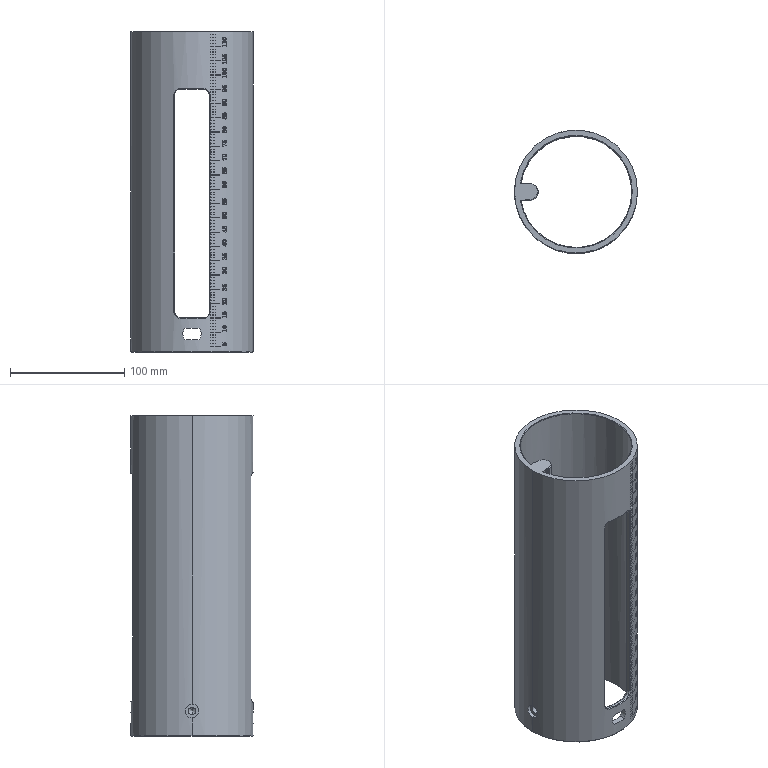Part | STEP file | PN_0010 Magazine clip | 1 solid | 1268 faces | box 107.5 x 107.5 x 280 mm | volume 444439 mm3 | plane 542 | spline 509 | cylinder 205 | cone 12 | commonest cylinder face diameters 107.4 x156 107.5 x25 10 x8 2 x4 16 x4 1.5 x2